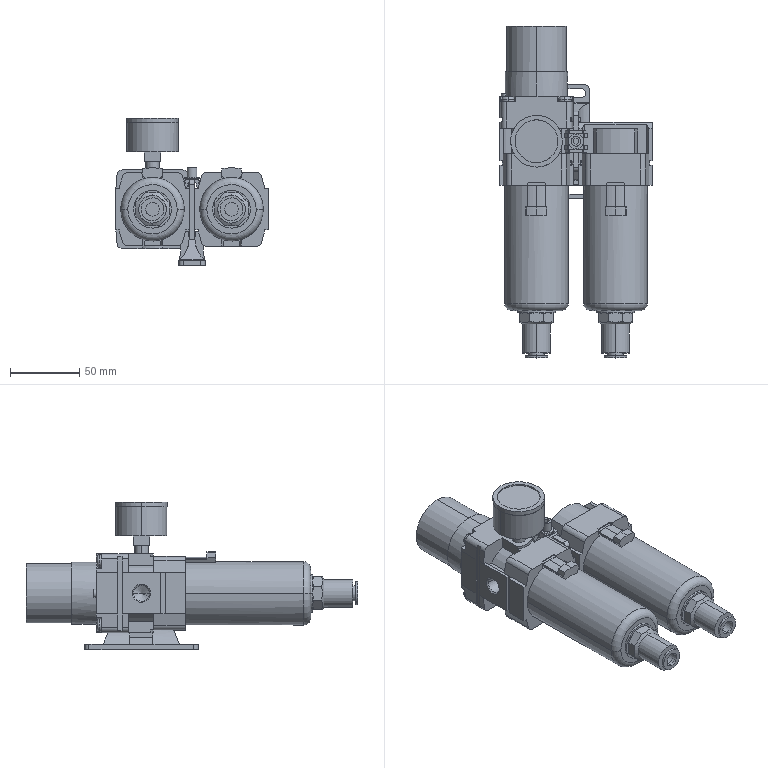Part | SolidWorks | features BaseBody 10 | 10 solids | 554 faces | box 110.2 x 240.3 x 107 mm | volume 709313 mm3 | plane 362 | cylinder 132 | cone 48 | torus 12 | commonest cylinder face diameters 8 x12 46 x10 3.242 x8 7 x8 9 x8 11.445 x8